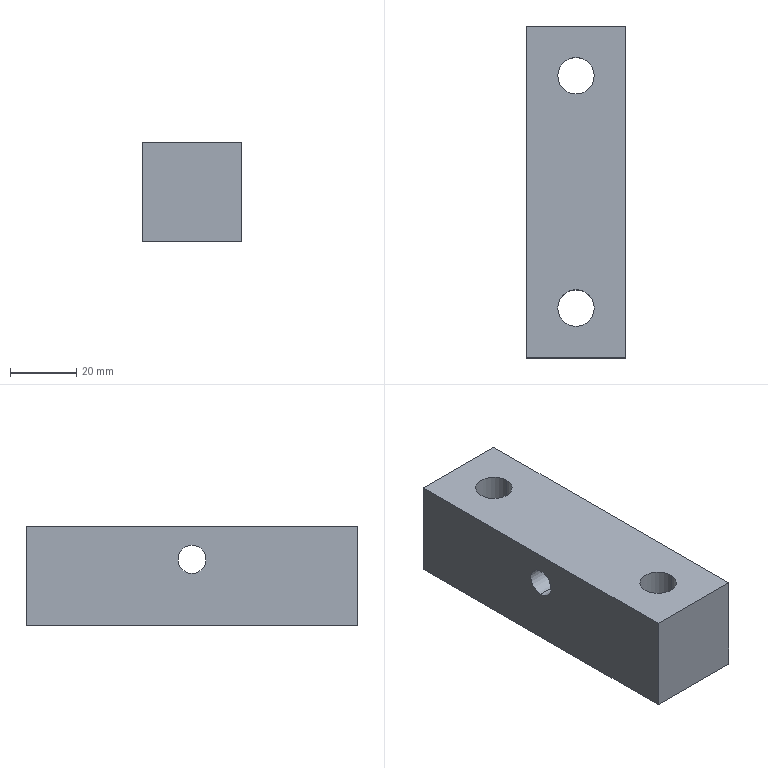Part | SolidWorks | features HoleWzd 2, Extrusion 1 | 1 solid | 18 faces | box 30 x 100 x 30 mm | volume 79088 mm3 | cylinder 10 | plane 8 | commonest cylinder face diameters 11 x4 18 x4 8.5 x2
STEP:
#1=CARTESIAN_POINT('',(15.,50.,0.75));
#2=VERTEX_POINT('',#1);
#3=CARTESIAN_POINT('',(15.,50.,9.25));
#4=VERTEX_POINT('',#3);
#5=CARTESIAN_POINT('',(15.,50.,5.));
#6=DIRECTION('',(-1.,0.,0.));
#7=DIRECTION('',(0.,0.,1.));
#8=AXIS2_PLACEMENT_3D('',#5,#6,#7);
#9=CIRCLE('',#8,4.25);
#10=EDGE_CURVE('',#2,#4,#9,.T.);
#11=ORIENTED_EDGE('',*,*,#10,.F.);
#12=CARTESIAN_POINT('',(-15.,50.,0.75));
#13=VERTEX_POINT('',#12);
#14=CARTESIAN_POINT('',(-15.,50.,0.75));
#15=DIRECTION('',(-1.,0.,0.));
#16=VECTOR('',#15,1000.);
#17=LINE('',#14,#16);
#18=EDGE_CURVE('',#2,#13,#17,.T.);
#19=ORIENTED_EDGE('',*,*,#18,.T.);
#20=CARTESIAN_POINT('',(-15.,50.,9.25));
#21=VERTEX_POINT('',#20);
#22=CARTESIAN_POINT('',(-15.,50.,5.));
#23=DIRECTION('',(-1.,0.,0.));
#24=DIRECTION('',(0.,0.,1.));
#25=AXIS2_PLACEMENT_3D('',#22,#23,#24);
#26=CIRCLE('',#25,4.25);
#27=EDGE_CURVE('',#13,#21,#26,.T.);
#28=ORIENTED_EDGE('',*,*,#27,.T.);
#29=CARTESIAN_POINT('',(-15.,50.,9.25));
#30=DIRECTION('',(-1.,0.,0.));
#31=VECTOR('',#30,1000.);
#32=LINE('',#29,#31);
#33=EDGE_CURVE('',#4,#21,#32,.T.);
#34=ORIENTED_EDGE('',*,*,#33,.F.);
#35=EDGE_LOOP('',(#11,#19,#28,#34));
#36=FACE_OUTER_BOUND('',#35,.T.);
#37=CARTESIAN_POINT('',(-15.,50.,5.));
#38=DIRECTION('',(-1.,0.,0.));
#39=DIRECTION('',(0.,0.,1.));
#40=AXIS2_PLACEMENT_3D('',#37,#38,#39);
#41=CYLINDRICAL_SURFACE('',#40,4.25);
#42=ADVANCED_FACE('',(#36),#41,.F.);
#43=CARTESIAN_POINT('',(9.,15.,-4.));
#44=VERTEX_POINT('',#43);
#45=CARTESIAN_POINT('',(-9.,15.,-4.));
#46=VERTEX_POINT('',#45);
#47=CARTESIAN_POINT('',(0.,15.,-4.));
#48=DIRECTION('',(0.,0.,-1.));
#49=DIRECTION('',(-1.,0.,0.));
#50=AXIS2_PLACEMENT_3D('',#47,#48,#49);
#51=CIRCLE('',#50,9.);
#52=EDGE_CURVE('',#44,#46,#51,.T.);
#53=ORIENTED_EDGE('',*,*,#52,.F.);
#54=CARTESIAN_POINT('',(9.,15.,-15.));
#55=VERTEX_POINT('',#54);
#56=CARTESIAN_POINT('',(9.,15.,-15.));
#57=DIRECTION('',(0.,0.,-1.));
#58=VECTOR('',#57,1000.);
#59=LINE('',#56,#58);
#60=EDGE_CURVE('',#44,#55,#59,.T.);
#61=ORIENTED_EDGE('',*,*,#60,.T.);
#62=CARTESIAN_POINT('',(-9.,15.,-15.));
#63=VERTEX_POINT('',#62);
#64=CARTESIAN_POINT('',(0.,15.,-15.));
#65=DIRECTION('',(0.,0.,-1.));
#66=DIRECTION('',(-1.,0.,0.));
#67=AXIS2_PLACEMENT_3D('',#64,#65,#66);
#68=CIRCLE('',#67,9.);
#69=EDGE_CURVE('',#55,#63,#68,.T.);
#70=ORIENTED_EDGE('',*,*,#69,.T.);
#71=CARTESIAN_POINT('',(-9.,15.,-15.));
#72=DIRECTION('',(0.,0.,-1.));
#73=VECTOR('',#72,1000.);
#74=LINE('',#71,#73);
#75=EDGE_CURVE('',#46,#63,#74,.T.);
#76=ORIENTED_EDGE('',*,*,#75,.F.);
#77=EDGE_LOOP('',(#53,#61,#70,#76));
#78=FACE_OUTER_BOUND('',#77,.T.);
#79=CARTESIAN_POINT('',(0.,15.,-15.));
#80=DIRECTION('',(0.,0.,-1.));
#81=DIRECTION('',(-1.,0.,0.));
#82=AXIS2_PLACEMENT_3D('',#79,#80,#81);
#83=CYLINDRICAL_SURFACE('',#82,9.);
#84=ADVANCED_FACE('',(#78),#83,.F.);
#85=CARTESIAN_POINT('',(5.5,15.,15.));
#86=VERTEX_POINT('',#85);
#87=CARTESIAN_POINT('',(-5.5,15.,15.));
#88=VERTEX_POINT('',#87);
#89=CARTESIAN_POINT('',(0.,15.,15.));
#90=DIRECTION('',(0.,0.,-1.));
#91=DIRECTION('',(-1.,0.,0.));
#92=AXIS2_PLACEMENT_3D('',#89,#90,#91);
#93=CIRCLE('',#92,5.5);
#94=EDGE_CURVE('',#86,#88,#93,.T.);
#95=ORIENTED_EDGE('',*,*,#94,.F.);
#96=CARTESIAN_POINT('',(5.5,15.,-4.));
#97=VERTEX_POINT('',#96);
#98=CARTESIAN_POINT('',(5.5,15.,-15.));
#99=DIRECTION('',(0.,0.,-1.));
#100=VECTOR('',#99,1000.);
#101=LINE('',#98,#100);
#102=EDGE_CURVE('',#86,#97,#101,.T.);
#103=ORIENTED_EDGE('',*,*,#102,.T.);
#104=CARTESIAN_POINT('',(-5.5,15.,-4.));
#105=VERTEX_POINT('',#104);
#106=CARTESIAN_POINT('',(0.,15.,-4.));
#107=DIRECTION('',(0.,0.,-1.));
#108=DIRECTION('',(-1.,0.,0.));
#109=AXIS2_PLACEMENT_3D('',#106,#107,#108);
#110=CIRCLE('',#109,5.5);
#111=EDGE_CURVE('',#97,#105,#110,.T.);
#112=ORIENTED_EDGE('',*,*,#111,.T.);
#113=CARTESIAN_POINT('',(-5.5,15.,-15.));
#114=DIRECTION('',(0.,0.,-1.));
#115=VECTOR('',#114,1000.);
#116=LINE('',#113,#115);
#117=EDGE_CURVE('',#88,#105,#116,.T.);
#118=ORIENTED_EDGE('',*,*,#117,.F.);
#119=EDGE_LOOP('',(#95,#103,#112,#118));
#120=FACE_OUTER_BOUND('',#119,.T.);
#121=CARTESIAN_POINT('',(0.,15.,-15.));
#122=DIRECTION('',(0.,0.,-1.));
#123=DIRECTION('',(-1.,0.,0.));
#124=AXIS2_PLACEMENT_3D('',#121,#122,#123);
#125=CYLINDRICAL_SURFACE('',#124,5.5);
#126=ADVANCED_FACE('',(#120),#125,.F.);
#127=CARTESIAN_POINT('',(9.,85.,-4.));
#128=VERTEX_POINT('',#127);
#129=CARTESIAN_POINT('',(-9.,85.,-4.));
#130=VERTEX_POINT('',#129);
#131=CARTESIAN_POINT('',(0.,85.,-4.));
#132=DIRECTION('',(0.,0.,-1.));
#133=DIRECTION('',(-1.,0.,0.));
#134=AXIS2_PLACEMENT_3D('',#131,#132,#133);
#135=CIRCLE('',#134,9.);
#136=EDGE_CURVE('',#128,#130,#135,.T.);
#137=ORIENTED_EDGE('',*,*,#136,.F.);
#138=CARTESIAN_POINT('',(9.,85.,-15.));
#139=VERTEX_POINT('',#138);
#140=CARTESIAN_POINT('',(9.,85.,-15.));
#141=DIRECTION('',(0.,0.,-1.));
#142=VECTOR('',#141,1000.);
#143=LINE('',#140,#142);
#144=EDGE_CURVE('',#128,#139,#143,.T.);
#145=ORIENTED_EDGE('',*,*,#144,.T.);
#146=CARTESIAN_POINT('',(-9.,85.,-15.));
#147=VERTEX_POINT('',#146);
#148=CARTESIAN_POINT('',(0.,85.,-15.));
#149=DIRECTION('',(0.,0.,-1.));
#150=DIRECTION('',(-1.,0.,0.));
#151=AXIS2_PLACEMENT_3D('',#148,#149,#150);
#152=CIRCLE('',#151,9.);
#153=EDGE_CURVE('',#139,#147,#152,.T.);
#154=ORIENTED_EDGE('',*,*,#153,.T.);
#155=CARTESIAN_POINT('',(-9.,85.,-15.));
#156=DIRECTION('',(0.,0.,-1.));
#157=VECTOR('',#156,1000.);
#158=LINE('',#155,#157);
#159=EDGE_CURVE('',#130,#147,#158,.T.);
#160=ORIENTED_EDGE('',*,*,#159,.F.);
#161=EDGE_LOOP('',(#137,#145,#154,#160));
#162=FACE_OUTER_BOUND('',#161,.T.);
#163=CARTESIAN_POINT('',(0.,85.,-15.));
#164=DIRECTION('',(0.,0.,-1.));
#165=DIRECTION('',(-1.,0.,0.));
#166=AXIS2_PLACEMENT_3D('',#163,#164,#165);
#167=CYLINDRICAL_SURFACE('',#166,9.);
#168=ADVANCED_FACE('',(#162),#167,.F.);
#169=CARTESIAN_POINT('',(5.5,85.,15.));
#170=VERTEX_POINT('',#169);
#171=CARTESIAN_POINT('',(-5.5,85.,15.));
#172=VERTEX_POINT('',#171);
#173=CARTESIAN_POINT('',(0.,85.,15.));
#174=DIRECTION('',(0.,0.,-1.));
#175=DIRECTION('',(-1.,0.,0.));
#176=AXIS2_PLACEMENT_3D('',#173,#174,#175);
#177=CIRCLE('',#176,5.5);
#178=EDGE_CURVE('',#170,#172,#177,.T.);
#179=ORIENTED_EDGE('',*,*,#178,.F.);
#180=CARTESIAN_POINT('',(5.5,85.,-4.));
#181=VERTEX_POINT('',#180);
#182=CARTESIAN_POINT('',(5.5,85.,-15.));
#183=DIRECTION('',(0.,0.,-1.));
#184=VECTOR('',#183,1000.);
#185=LINE('',#182,#184);
#186=EDGE_CURVE('',#170,#181,#185,.T.);
#187=ORIENTED_EDGE('',*,*,#186,.T.);
#188=CARTESIAN_POINT('',(-5.5,85.,-4.));
#189=VERTEX_POINT('',#188);
#190=CARTESIAN_POINT('',(0.,85.,-4.));
#191=DIRECTION('',(0.,0.,-1.));
#192=DIRECTION('',(-1.,0.,0.));
#193=AXIS2_PLACEMENT_3D('',#190,#191,#192);
#194=CIRCLE('',#193,5.5);
#195=EDGE_CURVE('',#181,#189,#194,.T.);
#196=ORIENTED_EDGE('',*,*,#195,.T.);
#197=CARTESIAN_POINT('',(-5.5,85.,-15.));
#198=DIRECTION('',(0.,0.,-1.));
#199=VECTOR('',#198,1000.);
#200=LINE('',#197,#199);
#201=EDGE_CURVE('',#172,#189,#200,.T.);
#202=ORIENTED_EDGE('',*,*,#201,.F.);
#203=EDGE_LOOP('',(#179,#187,#196,#202));
#204=FACE_OUTER_BOUND('',#203,.T.);
#205=CARTESIAN_POINT('',(0.,85.,-15.));
#206=DIRECTION('',(0.,0.,-1.));
#207=DIRECTION('',(-1.,0.,0.));
#208=AXIS2_PLACEMENT_3D('',#205,#206,#207);
#209=CYLINDRICAL_SURFACE('',#208,5.5);
#210=ADVANCED_FACE('',(#204),#209,.F.);
#211=CARTESIAN_POINT('',(15.,50.,5.));
#212=DIRECTION('',(-1.,0.,0.));
#213=DIRECTION('',(0.,0.,1.));
#214=AXIS2_PLACEMENT_3D('',#211,#212,#213);
#215=CIRCLE('',#214,4.25);
#216=EDGE_CURVE('',#4,#2,#215,.T.);
#217=ORIENTED_EDGE('',*,*,#216,.T.);
#218=ORIENTED_EDGE('',*,*,#10,.T.);
#219=EDGE_LOOP('',(#217,#218));
#220=FACE_BOUND('',#219,.T.);
#221=CARTESIAN_POINT('',(15.,0.,15.));
#222=VERTEX_POINT('',#221);
#223=CARTESIAN_POINT('',(15.,0.,-15.));
#224=VERTEX_POINT('',#223);
#225=CARTESIAN_POINT('',(15.,0.,15.));
#226=DIRECTION('',(0.,0.,-1.));
#227=VECTOR('',#226,1000.);
#228=LINE('',#225,#227);
#229=EDGE_CURVE('',#222,#224,#228,.T.);
#230=ORIENTED_EDGE('',*,*,#229,.T.);
#231=CARTESIAN_POINT('',(15.,100.,-15.));
#232=VERTEX_POINT('',#231);
#233=CARTESIAN_POINT('',(15.,100.,-15.));
#234=DIRECTION('',(0.,-1.,0.));
#235=VECTOR('',#234,1000.);
#236=LINE('',#233,#235);
#237=EDGE_CURVE('',#232,#224,#236,.T.);
#238=ORIENTED_EDGE('',*,*,#237,.F.);
#239=CARTESIAN_POINT('',(15.,100.,15.));
#240=VERTEX_POINT('',#239);
#241=CARTESIAN_POINT('',(15.,100.,15.));
#242=DIRECTION('',(0.,0.,-1.));
#243=VECTOR('',#242,1000.);
#244=LINE('',#241,#243);
#245=EDGE_CURVE('',#240,#232,#244,.T.);
#246=ORIENTED_EDGE('',*,*,#245,.F.);
#247=CARTESIAN_POINT('',(15.,100.,15.));
#248=DIRECTION('',(0.,-1.,0.));
#249=VECTOR('',#248,1000.);
#250=LINE('',#247,#249);
#251=EDGE_CURVE('',#240,#222,#250,.T.);
#252=ORIENTED_EDGE('',*,*,#251,.T.);
#253=EDGE_LOOP('',(#230,#238,#246,#252));
#254=FACE_OUTER_BOUND('',#253,.T.);
#255=CARTESIAN_POINT('',(15.,100.,15.));
#256=DIRECTION('',(-1.,0.,0.));
#257=DIRECTION('',(0.,0.,1.));
#258=AXIS2_PLACEMENT_3D('',#255,#256,#257);
#259=PLANE('',#258);
#260=ADVANCED_FACE('',(#220,#254),#259,.F.);
#261=CARTESIAN_POINT('',(0.,15.,-15.));
#262=DIRECTION('',(0.,0.,-1.));
#263=DIRECTION('',(-1.,0.,0.));
#264=AXIS2_PLACEMENT_3D('',#261,#262,#263);
#265=CIRCLE('',#264,9.);
#266=EDGE_CURVE('',#63,#55,#265,.T.);
#267=ORIENTED_EDGE('',*,*,#266,.F.);
#268=ORIENTED_EDGE('',*,*,#69,.F.);
#269=EDGE_LOOP('',(#267,#268));
#270=FACE_BOUND('',#269,.T.);
#271=CARTESIAN_POINT('',(0.,85.,-15.));
#272=DIRECTION('',(0.,0.,-1.));
#273=DIRECTION('',(-1.,0.,0.));
#274=AXIS2_PLACEMENT_3D('',#271,#272,#273);
#275=CIRCLE('',#274,9.);
#276=EDGE_CURVE('',#147,#139,#275,.T.);
#277=ORIENTED_EDGE('',*,*,#276,.F.);
#278=ORIENTED_EDGE('',*,*,#153,.F.);
#279=EDGE_LOOP('',(#277,#278));
#280=FACE_BOUND('',#279,.T.);
#281=CARTESIAN_POINT('',(-15.,0.,-15.));
#282=VERTEX_POINT('',#281);
#283=CARTESIAN_POINT('',(-15.,0.,-15.));
#284=DIRECTION('',(-1.,0.,0.));
#285=VECTOR('',#284,1000.);
#286=LINE('',#283,#285);
#287=EDGE_CURVE('',#224,#282,#286,.T.);
#288=ORIENTED_EDGE('',*,*,#287,.T.);
#289=CARTESIAN_POINT('',(-15.,100.,-15.));
#290=VERTEX_POINT('',#289);
#291=CARTESIAN_POINT('',(-15.,100.,-15.));
#292=DIRECTION('',(0.,-1.,0.));
#293=VECTOR('',#292,1000.);
#294=LINE('',#291,#293);
#295=EDGE_CURVE('',#290,#282,#294,.T.);
#296=ORIENTED_EDGE('',*,*,#295,.F.);
#297=CARTESIAN_POINT('',(-15.,100.,-15.));
#298=DIRECTION('',(-1.,0.,0.));
#299=VECTOR('',#298,1000.);
#300=LINE('',#297,#299);
#301=EDGE_CURVE('',#232,#290,#300,.T.);
#302=ORIENTED_EDGE('',*,*,#301,.F.);
#303=ORIENTED_EDGE('',*,*,#237,.T.);
#304=EDGE_LOOP('',(#288,#296,#302,#303));
#305=FACE_OUTER_BOUND('',#304,.T.);
#306=CARTESIAN_POINT('',(-15.,100.,-15.));
#307=DIRECTION('',(0.,0.,1.));
#308=DIRECTION('',(1.,0.,0.));
#309=AXIS2_PLACEMENT_3D('',#306,#307,#308);
#310=PLANE('',#309);
#311=ADVANCED_FACE('',(#270,#280,#305),#310,.F.);
#312=CARTESIAN_POINT('',(-15.,50.,5.));
#313=DIRECTION('',(-1.,0.,0.));
#314=DIRECTION('',(0.,0.,1.));
#315=AXIS2_PLACEMENT_3D('',#312,#313,#314);
#316=CIRCLE('',#315,4.25);
#317=EDGE_CURVE('',#21,#13,#316,.T.);
#318=ORIENTED_EDGE('',*,*,#317,.F.);
#319=ORIENTED_EDGE('',*,*,#27,.F.);
#320=EDGE_LOOP('',(#318,#319));
#321=FACE_BOUND('',#320,.T.);
#322=CARTESIAN_POINT('',(-15.,0.,15.));
#323=VERTEX_POINT('',#322);
#324=CARTESIAN_POINT('',(-15.,0.,15.));
#325=DIRECTION('',(0.,0.,1.));
#326=VECTOR('',#325,1000.);
#327=LINE('',#324,#326);
#328=EDGE_CURVE('',#282,#323,#327,.T.);
#329=ORIENTED_EDGE('',*,*,#328,.T.);
#330=CARTESIAN_POINT('',(-15.,100.,15.));
#331=VERTEX_POINT('',#330);
#332=CARTESIAN_POINT('',(-15.,100.,15.));
#333=DIRECTION('',(0.,-1.,0.));
#334=VECTOR('',#333,1000.);
#335=LINE('',#332,#334);
#336=EDGE_CURVE('',#331,#323,#335,.T.);
#337=ORIENTED_EDGE('',*,*,#336,.F.);
#338=CARTESIAN_POINT('',(-15.,100.,15.));
#339=DIRECTION('',(0.,0.,1.));
#340=VECTOR('',#339,1000.);
#341=LINE('',#338,#340);
#342=EDGE_CURVE('',#290,#331,#341,.T.);
#343=ORIENTED_EDGE('',*,*,#342,.F.);
#344=ORIENTED_EDGE('',*,*,#295,.T.);
#345=EDGE_LOOP('',(#329,#337,#343,#344));
#346=FACE_OUTER_BOUND('',#345,.T.);
#347=CARTESIAN_POINT('',(-15.,100.,15.));
#348=DIRECTION('',(1.,0.,0.));
#349=DIRECTION('',(0.,0.,-1.));
#350=AXIS2_PLACEMENT_3D('',#347,#348,#349);
#351=PLANE('',#350);
#352=ADVANCED_FACE('',(#321,#346),#351,.F.);
#353=CARTESIAN_POINT('',(0.,15.,15.));
#354=DIRECTION('',(0.,0.,-1.));
#355=DIRECTION('',(-1.,0.,0.));
#356=AXIS2_PLACEMENT_3D('',#353,#354,#355);
#357=CIRCLE('',#356,5.5);
#358=EDGE_CURVE('',#88,#86,#357,.T.);
#359=ORIENTED_EDGE('',*,*,#358,.T.);
#360=ORIENTED_EDGE('',*,*,#94,.T.);
#361=EDGE_LOOP('',(#359,#360));
#362=FACE_BOUND('',#361,.T.);
#363=CARTESIAN_POINT('',(0.,85.,15.));
#364=DIRECTION('',(0.,0.,-1.));
#365=DIRECTION('',(-1.,0.,0.));
#366=AXIS2_PLACEMENT_3D('',#363,#364,#365);
#367=CIRCLE('',#366,5.5);
#368=EDGE_CURVE('',#172,#170,#367,.T.);
#369=ORIENTED_EDGE('',*,*,#368,.T.);
#370=ORIENTED_EDGE('',*,*,#178,.T.);
#371=EDGE_LOOP('',(#369,#370));
#372=FACE_BOUND('',#371,.T.);
#373=CARTESIAN_POINT('',(-15.,0.,15.));
#374=DIRECTION('',(1.,0.,0.));
#375=VECTOR('',#374,1000.);
#376=LINE('',#373,#375);
#377=EDGE_CURVE('',#323,#222,#376,.T.);
#378=ORIENTED_EDGE('',*,*,#377,.T.);
#379=ORIENTED_EDGE('',*,*,#251,.F.);
#380=CARTESIAN_POINT('',(-15.,100.,15.));
#381=DIRECTION('',(1.,0.,0.));
#382=VECTOR('',#381,1000.);
#383=LINE('',#380,#382);
#384=EDGE_CURVE('',#331,#240,#383,.T.);
#385=ORIENTED_EDGE('',*,*,#384,.F.);
#386=ORIENTED_EDGE('',*,*,#336,.T.);
#387=EDGE_LOOP('',(#378,#379,#385,#386));
#388=FACE_OUTER_BOUND('',#387,.T.);
#389=CARTESIAN_POINT('',(-15.,100.,15.));
#390=DIRECTION('',(0.,0.,-1.));
#391=DIRECTION('',(-1.,0.,0.));
#392=AXIS2_PLACEMENT_3D('',#389,#390,#391);
#393=PLANE('',#392);
#394=ADVANCED_FACE('',(#362,#372,#388),#393,.F.);
#395=ORIENTED_EDGE('',*,*,#245,.T.);
#396=ORIENTED_EDGE('',*,*,#301,.T.);
#397=ORIENTED_EDGE('',*,*,#342,.T.);
#398=ORIENTED_EDGE('',*,*,#384,.T.);
#399=EDGE_LOOP('',(#395,#396,#397,#398));
#400=FACE_OUTER_BOUND('',#399,.T.);
#401=CARTESIAN_POINT('',(0.,100.,0.));
#402=DIRECTION('',(0.,-1.,0.));
#403=DIRECTION('',(0.,0.,-1.));
#404=AXIS2_PLACEMENT_3D('',#401,#402,#403);
#405=PLANE('',#404);
#406=ADVANCED_FACE('',(#400),#405,.F.);
#407=ORIENTED_EDGE('',*,*,#229,.F.);
#408=ORIENTED_EDGE('',*,*,#377,.F.);
#409=ORIENTED_EDGE('',*,*,#328,.F.);
#410=ORIENTED_EDGE('',*,*,#287,.F.);
#411=EDGE_LOOP('',(#407,#408,#409,#410));
#412=FACE_OUTER_BOUND('',#411,.T.);
#413=CARTESIAN_POINT('',(0.,0.,0.));
#414=DIRECTION('',(0.,-1.,0.));
#415=DIRECTION('',(0.,0.,-1.));
#416=AXIS2_PLACEMENT_3D('',#413,#414,#415);
#417=PLANE('',#416);
#418=ADVANCED_FACE('',(#412),#417,.T.);
#419=ORIENTED_EDGE('',*,*,#186,.F.);
#420=ORIENTED_EDGE('',*,*,#368,.F.);
#421=ORIENTED_EDGE('',*,*,#201,.T.);
#422=CARTESIAN_POINT('',(0.,85.,-4.));
#423=DIRECTION('',(0.,0.,-1.));
#424=DIRECTION('',(-1.,0.,0.));
#425=AXIS2_PLACEMENT_3D('',#422,#423,#424);
#426=CIRCLE('',#425,5.5);
#427=EDGE_CURVE('',#189,#181,#426,.T.);
#428=ORIENTED_EDGE('',*,*,#427,.T.);
#429=EDGE_LOOP('',(#419,#420,#421,#428));
#430=FACE_OUTER_BOUND('',#429,.T.);
#431=CARTESIAN_POINT('',(0.,85.,-15.));
#432=DIRECTION('',(0.,0.,-1.));
#433=DIRECTION('',(-1.,0.,0.));
#434=AXIS2_PLACEMENT_3D('',#431,#432,#433);
#435=CYLINDRICAL_SURFACE('',#434,5.5);
#436=ADVANCED_FACE('',(#430),#435,.F.);
#437=ORIENTED_EDGE('',*,*,#427,.F.);
#438=ORIENTED_EDGE('',*,*,#195,.F.);
#439=EDGE_LOOP('',(#437,#438));
#440=FACE_BOUND('',#439,.T.);
#441=CARTESIAN_POINT('',(0.,85.,-4.));
#442=DIRECTION('',(0.,0.,-1.));
#443=DIRECTION('',(-1.,0.,0.));
#444=AXIS2_PLACEMENT_3D('',#441,#442,#443);
#445=CIRCLE('',#444,9.);
#446=EDGE_CURVE('',#130,#128,#445,.T.);
#447=ORIENTED_EDGE('',*,*,#446,.T.);
#448=ORIENTED_EDGE('',*,*,#136,.T.);
#449=EDGE_LOOP('',(#447,#448));
#450=FACE_OUTER_BOUND('',#449,.T.);
#451=CARTESIAN_POINT('',(5.5,85.,-4.));
#452=DIRECTION('',(0.,0.,1.));
#453=DIRECTION('',(1.,0.,0.));
#454=AXIS2_PLACEMENT_3D('',#451,#452,#453);
#455=PLANE('',#454);
#456=ADVANCED_FACE('',(#440,#450),#455,.F.);
#457=ORIENTED_EDGE('',*,*,#144,.F.);
#458=ORIENTED_EDGE('',*,*,#446,.F.);
#459=ORIENTED_EDGE('',*,*,#159,.T.);
#460=ORIENTED_EDGE('',*,*,#276,.T.);
#461=EDGE_LOOP('',(#457,#458,#459,#460));
#462=FACE_OUTER_BOUND('',#461,.T.);
#463=CARTESIAN_POINT('',(0.,85.,-15.));
#464=DIRECTION('',(0.,0.,-1.));
#465=DIRECTION('',(-1.,0.,0.));
#466=AXIS2_PLACEMENT_3D('',#463,#464,#465);
#467=CYLINDRICAL_SURFACE('',#466,9.);
#468=ADVANCED_FACE('',(#462),#467,.F.);
#469=ORIENTED_EDGE('',*,*,#102,.F.);
#470=ORIENTED_EDGE('',*,*,#358,.F.);
#471=ORIENTED_EDGE('',*,*,#117,.T.);
#472=CARTESIAN_POINT('',(0.,15.,-4.));
#473=DIRECTION('',(0.,0.,-1.));
#474=DIRECTION('',(-1.,0.,0.));
#475=AXIS2_PLACEMENT_3D('',#472,#473,#474);
#476=CIRCLE('',#475,5.5);
#477=EDGE_CURVE('',#105,#97,#476,.T.);
#478=ORIENTED_EDGE('',*,*,#477,.T.);
#479=EDGE_LOOP('',(#469,#470,#471,#478));
#480=FACE_OUTER_BOUND('',#479,.T.);
#481=CARTESIAN_POINT('',(0.,15.,-15.));
#482=DIRECTION('',(0.,0.,-1.));
#483=DIRECTION('',(-1.,0.,0.));
#484=AXIS2_PLACEMENT_3D('',#481,#482,#483);
#485=CYLINDRICAL_SURFACE('',#484,5.5);
#486=ADVANCED_FACE('',(#480),#485,.F.);
#487=ORIENTED_EDGE('',*,*,#477,.F.);
#488=ORIENTED_EDGE('',*,*,#111,.F.);
#489=EDGE_LOOP('',(#487,#488));
#490=FACE_BOUND('',#489,.T.);
#491=CARTESIAN_POINT('',(0.,15.,-4.));
#492=DIRECTION('',(0.,0.,-1.));
#493=DIRECTION('',(-1.,0.,0.));
#494=AXIS2_PLACEMENT_3D('',#491,#492,#493);
#495=CIRCLE('',#494,9.);
#496=EDGE_CURVE('',#46,#44,#495,.T.);
#497=ORIENTED_EDGE('',*,*,#496,.T.);
#498=ORIENTED_EDGE('',*,*,#52,.T.);
#499=EDGE_LOOP('',(#497,#498));
#500=FACE_OUTER_BOUND('',#499,.T.);
#501=CARTESIAN_POINT('',(5.5,15.,-4.));
#502=DIRECTION('',(0.,0.,1.));
#503=DIRECTION('',(1.,0.,0.));
#504=AXIS2_PLACEMENT_3D('',#501,#502,#503);
#505=PLANE('',#504);
#506=ADVANCED_FACE('',(#490,#500),#505,.F.);
#507=ORIENTED_EDGE('',*,*,#60,.F.);
#508=ORIENTED_EDGE('',*,*,#496,.F.);
#509=ORIENTED_EDGE('',*,*,#75,.T.);
#510=ORIENTED_EDGE('',*,*,#266,.T.);
#511=EDGE_LOOP('',(#507,#508,#509,#510));
#512=FACE_OUTER_BOUND('',#511,.T.);
#513=CARTESIAN_POINT('',(0.,15.,-15.));
#514=DIRECTION('',(0.,0.,-1.));
#515=DIRECTION('',(-1.,0.,0.));
#516=AXIS2_PLACEMENT_3D('',#513,#514,#515);
#517=CYLINDRICAL_SURFACE('',#516,9.);
#518=ADVANCED_FACE('',(#512),#517,.F.);
#519=ORIENTED_EDGE('',*,*,#18,.F.);
#520=ORIENTED_EDGE('',*,*,#216,.F.);
#521=ORIENTED_EDGE('',*,*,#33,.T.);
#522=ORIENTED_EDGE('',*,*,#317,.T.);
#523=EDGE_LOOP('',(#519,#520,#521,#522));
#524=FACE_OUTER_BOUND('',#523,.T.);
#525=CARTESIAN_POINT('',(-15.,50.,5.));
#526=DIRECTION('',(-1.,0.,0.));
#527=DIRECTION('',(0.,0.,1.));
#528=AXIS2_PLACEMENT_3D('',#525,#526,#527);
#529=CYLINDRICAL_SURFACE('',#528,4.25);
#530=ADVANCED_FACE('',(#524),#529,.F.);
#531=CLOSED_SHELL('',(#42,#84,#126,#168,#210,#260,#311,#352,#394,#406,#418,#436,#456,#468,#486,#506,#518,#530));
#532=MANIFOLD_SOLID_BREP('',#531);
#533=CARTESIAN_POINT('',(0.,0.,0.));
#534=DIRECTION('',(0.,0.,1.));
#535=DIRECTION('',(1.,0.,0.));
#536=AXIS2_PLACEMENT_3D('',#533,#534,#535);
#537=(LENGTH_UNIT()NAMED_UNIT(*)SI_UNIT(.MILLI.,.METRE.));
#538=UNCERTAINTY_MEASURE_WITH_UNIT(LENGTH_MEASURE(0.00001),#537,'','');
#539=(NAMED_UNIT(*)PLANE_ANGLE_UNIT()SI_UNIT($,.RADIAN.));
#540=(NAMED_UNIT(*)SI_UNIT($,.STERADIAN.)SOLID_ANGLE_UNIT());
#541=(GEOMETRIC_REPRESENTATION_CONTEXT(3)GLOBAL_UNCERTAINTY_ASSIGNED_CONTEXT((#538))GLOBAL_UNIT_ASSIGNED_CONTEXT((#537,#539,#540))REPRESENTATION_CONTEXT('',''));
#542=ADVANCED_BREP_SHAPE_REPRESENTATION('',(#532,#536),#541);